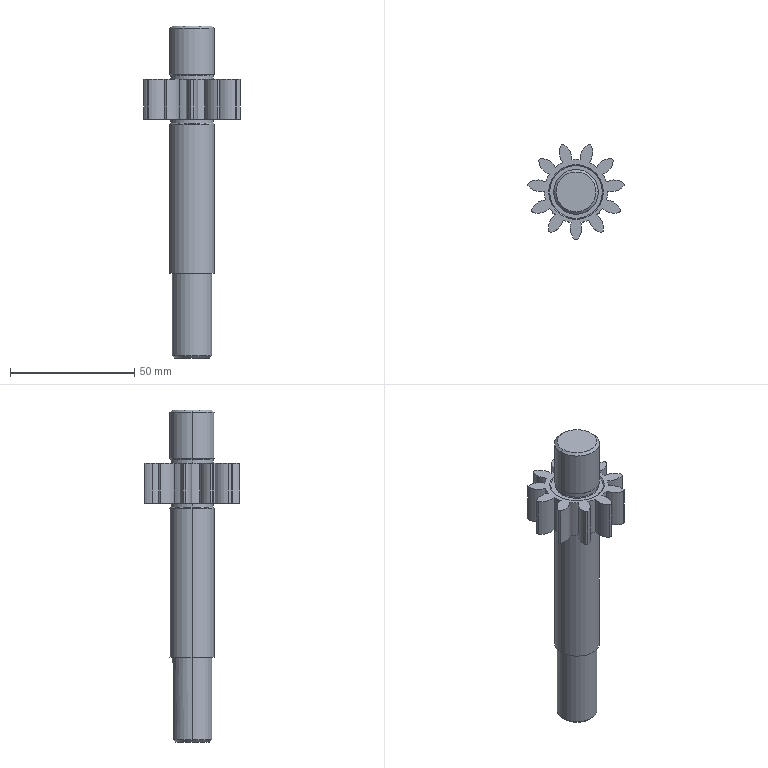Part | SolidWorks | features ICE 4, Chamfer 1, Extrusion 1, MirrorPattern 1, RevCut 1 | 1 solid | 88 faces | box 38.724 x 38.336 x 133.5 mm | volume 40115 mm3 | cylinder 59 | cone 13 | plane 12 | torus 4 | commonest cylinder face diameters 13.2 x26 25.498 x11 39 x11 17.179 x4 18 x4 16 x2